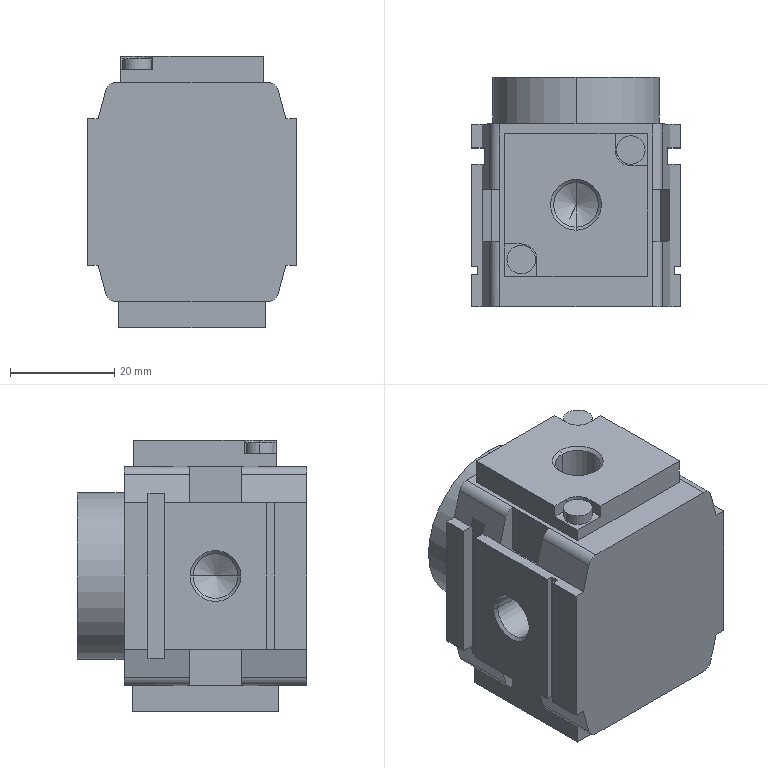Part | STEP file | 25A-AR20K-01B-D-Part-3 | 1 solid | 157 faces | box 40 x 44 x 52 mm | volume 66870 mm3 | plane 117 | cylinder 28 | cone 12 | commonest cylinder face diameters 8.566 x6 4 x4 5.5 x4 6 x2 27.5 x2 32 x2